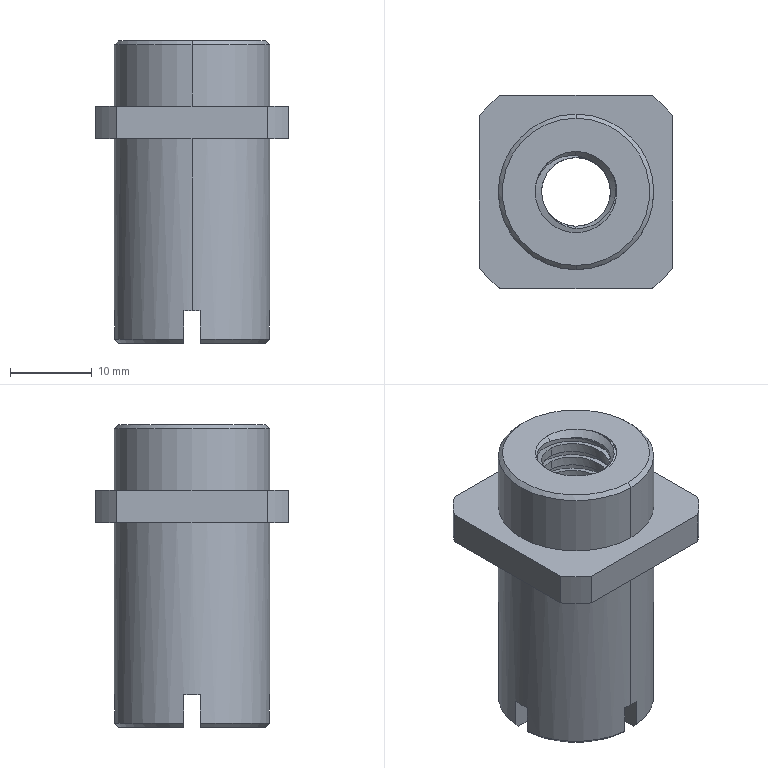Part | NX | features BREP 1 | 1 solid | 66 faces | box 23.7 x 23.7 x 37 mm | volume 6865 mm3 | plane 24 | cylinder 24 | cone 16 | spline 2 | commonest cylinder face diameters 8.4 x13 19 x4 30 x4 14 x2 10 x1